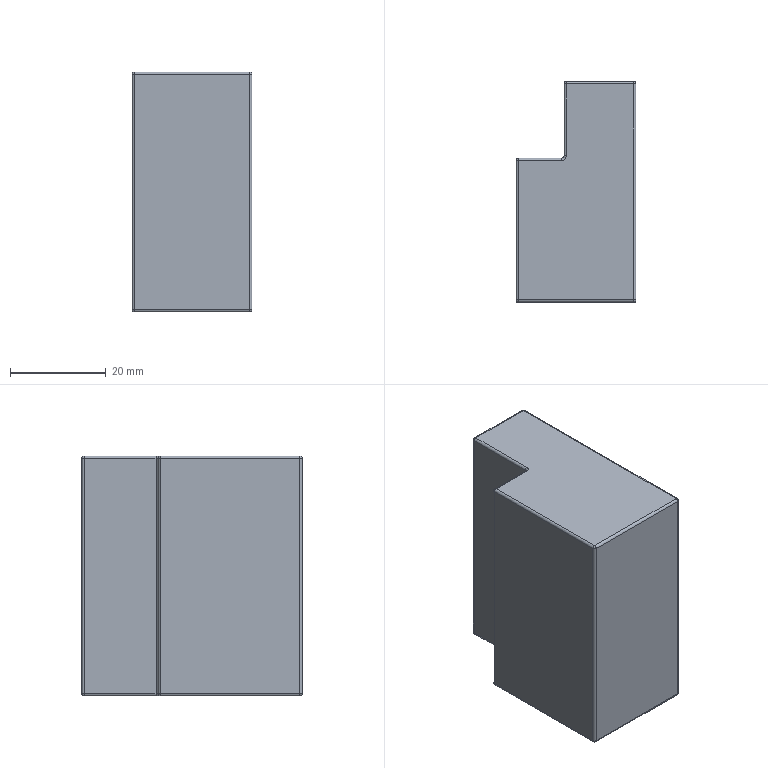Part | STEP file | GLSJ-10-43_default | 1 solid | 50 faces | box 25 x 46 x 50 mm | volume 48561 mm3 | cylinder 24 | sphere 10 | plane 8 | cone 6 | torus 2 | commonest cylinder face diameters 1 x18 5 x6